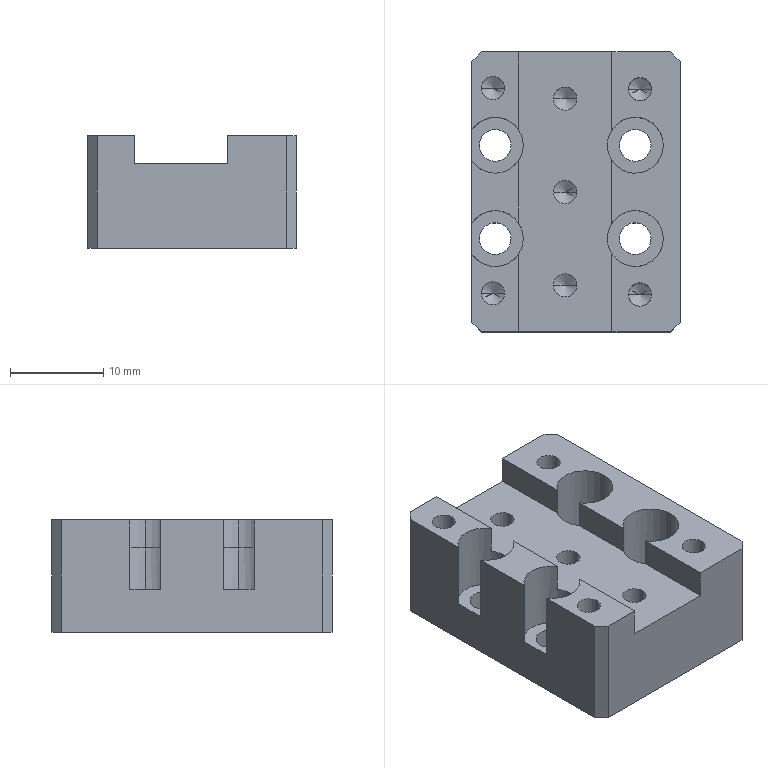Part | NX | features BREP 1 | 1 solid | 84 faces | box 22.3 x 30 x 12 mm | volume 5809 mm3 | cylinder 42 | plane 24 | cone 18 | commonest cylinder face diameters 2.5 x26 3.4 x8 6 x8